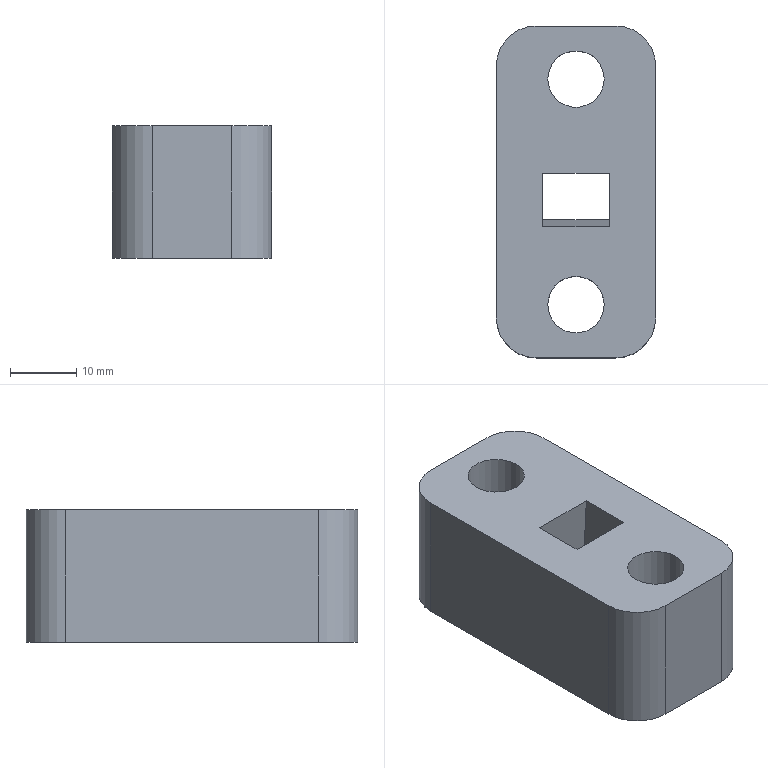Part | STEP file | solid 90 | 1 solid | 28 faces | box 24 x 50 x 20 mm | volume 17760 mm3 | plane 16 | cylinder 8 | other 4 | commonest cylinder face diameters 12 x4 8.5 x2 14 x2